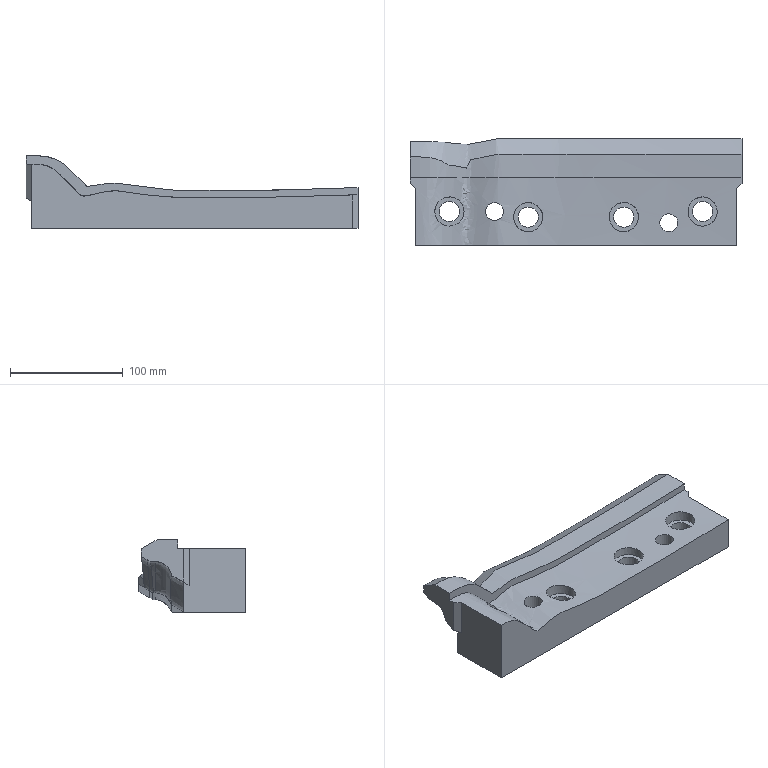Part | NX | features solid 2 | 1 solid | 48 faces | box 295 x 94.751 x 64.552 mm | volume 734783 mm3 | spline 24 | plane 14 | cylinder 10 | commonest cylinder face diameters 18 x4 26 x4 16 x2